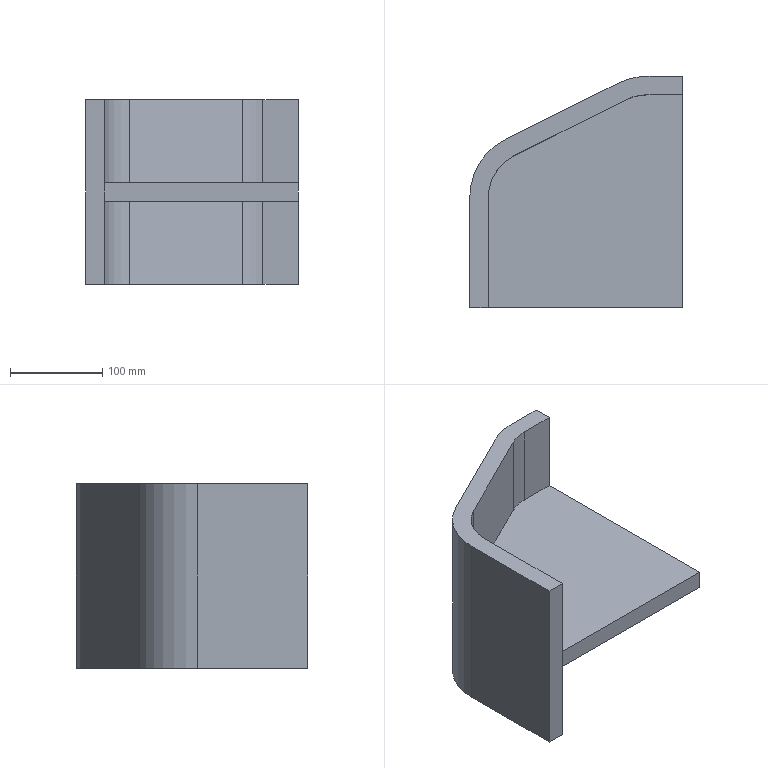Part | SolidWorks | features Extrusion 1, ICE 1 | 2 solids | 23 faces | box 230 x 250 x 200 mm | volume 2385457 mm3 | plane 17 | cylinder 6 | commonest cylinder face diameters 100 x4 140 x2
STEP:
#1=CARTESIAN_POINT('',(0.,119.098,0.));
#2=VERTEX_POINT('',#1);
#3=CARTESIAN_POINT('',(0.,0.,0.));
#4=VERTEX_POINT('',#3);
#5=CARTESIAN_POINT('',(0.,0.,0.));
#6=DIRECTION('',(0.,-1.,0.));
#7=VECTOR('',#6,1000.);
#8=LINE('',#5,#7);
#9=EDGE_CURVE('',#2,#4,#8,.T.);
#10=ORIENTED_EDGE('',*,*,#9,.T.);
#11=CARTESIAN_POINT('',(0.,0.,20.));
#12=VERTEX_POINT('',#11);
#13=CARTESIAN_POINT('',(0.,0.,20.));
#14=DIRECTION('',(0.,0.,-1.));
#15=VECTOR('',#14,1000.);
#16=LINE('',#13,#15);
#17=EDGE_CURVE('',#12,#4,#16,.T.);
#18=ORIENTED_EDGE('',*,*,#17,.F.);
#19=CARTESIAN_POINT('',(0.,119.098,20.));
#20=VERTEX_POINT('',#19);
#21=CARTESIAN_POINT('',(0.,0.,20.));
#22=DIRECTION('',(0.,-1.,0.));
#23=VECTOR('',#22,1000.);
#24=LINE('',#21,#23);
#25=EDGE_CURVE('',#20,#12,#24,.T.);
#26=ORIENTED_EDGE('',*,*,#25,.F.);
#27=CARTESIAN_POINT('',(0.,119.098,20.));
#28=DIRECTION('',(0.,0.,-1.));
#29=VECTOR('',#28,1000.);
#30=LINE('',#27,#29);
#31=EDGE_CURVE('',#20,#2,#30,.T.);
#32=ORIENTED_EDGE('',*,*,#31,.T.);
#33=EDGE_LOOP('',(#10,#18,#26,#32));
#34=FACE_OUTER_BOUND('',#33,.T.);
#35=CARTESIAN_POINT('',(0.,0.,20.));
#36=DIRECTION('',(1.,0.,0.));
#37=DIRECTION('',(0.,0.,-1.));
#38=AXIS2_PLACEMENT_3D('',#35,#36,#37);
#39=PLANE('',#38);
#40=ADVANCED_FACE('',(#34),#39,.F.);
#41=CARTESIAN_POINT('',(210.,0.,0.));
#42=VERTEX_POINT('',#41);
#43=CARTESIAN_POINT('',(0.,0.,0.));
#44=DIRECTION('',(1.,0.,0.));
#45=VECTOR('',#44,1000.);
#46=LINE('',#43,#45);
#47=EDGE_CURVE('',#4,#42,#46,.T.);
#48=ORIENTED_EDGE('',*,*,#47,.T.);
#49=CARTESIAN_POINT('',(210.,0.,20.));
#50=VERTEX_POINT('',#49);
#51=CARTESIAN_POINT('',(210.,0.,20.));
#52=DIRECTION('',(0.,0.,-1.));
#53=VECTOR('',#52,1000.);
#54=LINE('',#51,#53);
#55=EDGE_CURVE('',#50,#42,#54,.T.);
#56=ORIENTED_EDGE('',*,*,#55,.F.);
#57=CARTESIAN_POINT('',(0.,0.,20.));
#58=DIRECTION('',(1.,0.,0.));
#59=VECTOR('',#58,1000.);
#60=LINE('',#57,#59);
#61=EDGE_CURVE('',#12,#50,#60,.T.);
#62=ORIENTED_EDGE('',*,*,#61,.F.);
#63=ORIENTED_EDGE('',*,*,#17,.T.);
#64=EDGE_LOOP('',(#48,#56,#62,#63));
#65=FACE_OUTER_BOUND('',#64,.T.);
#66=CARTESIAN_POINT('',(0.,0.,20.));
#67=DIRECTION('',(0.,1.,0.));
#68=DIRECTION('',(0.,0.,1.));
#69=AXIS2_PLACEMENT_3D('',#66,#67,#68);
#70=PLANE('',#69);
#71=ADVANCED_FACE('',(#65),#70,.F.);
#72=CARTESIAN_POINT('',(210.,230.,0.));
#73=VERTEX_POINT('',#72);
#74=CARTESIAN_POINT('',(210.,230.,0.));
#75=DIRECTION('',(0.,1.,0.));
#76=VECTOR('',#75,1000.);
#77=LINE('',#74,#76);
#78=EDGE_CURVE('',#42,#73,#77,.T.);
#79=ORIENTED_EDGE('',*,*,#78,.T.);
#80=CARTESIAN_POINT('',(210.,230.,20.));
#81=VERTEX_POINT('',#80);
#82=CARTESIAN_POINT('',(210.,230.,20.));
#83=DIRECTION('',(0.,0.,-1.));
#84=VECTOR('',#83,1000.);
#85=LINE('',#82,#84);
#86=EDGE_CURVE('',#81,#73,#85,.T.);
#87=ORIENTED_EDGE('',*,*,#86,.F.);
#88=CARTESIAN_POINT('',(210.,230.,20.));
#89=DIRECTION('',(0.,1.,0.));
#90=VECTOR('',#89,1000.);
#91=LINE('',#88,#90);
#92=EDGE_CURVE('',#50,#81,#91,.T.);
#93=ORIENTED_EDGE('',*,*,#92,.F.);
#94=ORIENTED_EDGE('',*,*,#55,.T.);
#95=EDGE_LOOP('',(#79,#87,#93,#94));
#96=FACE_OUTER_BOUND('',#95,.T.);
#97=CARTESIAN_POINT('',(210.,230.,20.));
#98=DIRECTION('',(-1.,0.,0.));
#99=DIRECTION('',(0.,-1.,0.));
#100=AXIS2_PLACEMENT_3D('',#97,#98,#99);
#101=PLANE('',#100);
#102=ADVANCED_FACE('',(#96),#101,.F.);
#103=CARTESIAN_POINT('',(171.803,230.,0.));
#104=VERTEX_POINT('',#103);
#105=CARTESIAN_POINT('',(171.803,230.,0.));
#106=DIRECTION('',(-1.,0.,0.));
#107=VECTOR('',#106,1000.);
#108=LINE('',#105,#107);
#109=EDGE_CURVE('',#73,#104,#108,.T.);
#110=ORIENTED_EDGE('',*,*,#109,.T.);
#111=CARTESIAN_POINT('',(171.803,230.,20.));
#112=VERTEX_POINT('',#111);
#113=CARTESIAN_POINT('',(171.803,230.,20.));
#114=DIRECTION('',(0.,0.,-1.));
#115=VECTOR('',#114,1000.);
#116=LINE('',#113,#115);
#117=EDGE_CURVE('',#112,#104,#116,.T.);
#118=ORIENTED_EDGE('',*,*,#117,.F.);
#119=CARTESIAN_POINT('',(171.803,230.,20.));
#120=DIRECTION('',(-1.,0.,0.));
#121=VECTOR('',#120,1000.);
#122=LINE('',#119,#121);
#123=EDGE_CURVE('',#81,#112,#122,.T.);
#124=ORIENTED_EDGE('',*,*,#123,.F.);
#125=ORIENTED_EDGE('',*,*,#86,.T.);
#126=EDGE_LOOP('',(#110,#118,#124,#125));
#127=FACE_OUTER_BOUND('',#126,.T.);
#128=CARTESIAN_POINT('',(171.803,230.,20.));
#129=DIRECTION('',(0.,-1.,0.));
#130=DIRECTION('',(0.,0.,-1.));
#131=AXIS2_PLACEMENT_3D('',#128,#129,#130);
#132=PLANE('',#131);
#133=ADVANCED_FACE('',(#127),#132,.F.);
#134=CARTESIAN_POINT('',(149.443,224.721,0.));
#135=VERTEX_POINT('',#134);
#136=CARTESIAN_POINT('',(171.803,180.,0.));
#137=DIRECTION('',(0.,0.,1.));
#138=DIRECTION('',(-1.,0.,0.));
#139=AXIS2_PLACEMENT_3D('',#136,#137,#138);
#140=CIRCLE('',#139,50.);
#141=EDGE_CURVE('',#104,#135,#140,.T.);
#142=ORIENTED_EDGE('',*,*,#141,.T.);
#143=CARTESIAN_POINT('',(149.443,224.721,20.));
#144=VERTEX_POINT('',#143);
#145=CARTESIAN_POINT('',(149.443,224.721,20.));
#146=DIRECTION('',(0.,0.,-1.));
#147=VECTOR('',#146,1000.);
#148=LINE('',#145,#147);
#149=EDGE_CURVE('',#144,#135,#148,.T.);
#150=ORIENTED_EDGE('',*,*,#149,.F.);
#151=CARTESIAN_POINT('',(171.803,180.,20.));
#152=DIRECTION('',(0.,0.,1.));
#153=DIRECTION('',(-1.,0.,0.));
#154=AXIS2_PLACEMENT_3D('',#151,#152,#153);
#155=CIRCLE('',#154,50.);
#156=EDGE_CURVE('',#112,#144,#155,.T.);
#157=ORIENTED_EDGE('',*,*,#156,.F.);
#158=ORIENTED_EDGE('',*,*,#117,.T.);
#159=EDGE_LOOP('',(#142,#150,#157,#158));
#160=FACE_OUTER_BOUND('',#159,.T.);
#161=CARTESIAN_POINT('',(171.803,180.,20.));
#162=DIRECTION('',(0.,0.,-1.));
#163=DIRECTION('',(-1.,0.,0.));
#164=AXIS2_PLACEMENT_3D('',#161,#162,#163);
#165=CYLINDRICAL_SURFACE('',#164,50.);
#166=ADVANCED_FACE('',(#160),#165,.T.);
#167=CARTESIAN_POINT('',(27.639,163.82,0.));
#168=VERTEX_POINT('',#167);
#169=CARTESIAN_POINT('',(149.443,224.721,0.));
#170=DIRECTION('',(-0.8944,-0.4472,0.));
#171=VECTOR('',#170,1000.);
#172=LINE('',#169,#171);
#173=EDGE_CURVE('',#135,#168,#172,.T.);
#174=ORIENTED_EDGE('',*,*,#173,.T.);
#175=CARTESIAN_POINT('',(27.639,163.82,20.));
#176=VERTEX_POINT('',#175);
#177=CARTESIAN_POINT('',(27.639,163.82,20.));
#178=DIRECTION('',(0.,0.,-1.));
#179=VECTOR('',#178,1000.);
#180=LINE('',#177,#179);
#181=EDGE_CURVE('',#176,#168,#180,.T.);
#182=ORIENTED_EDGE('',*,*,#181,.F.);
#183=CARTESIAN_POINT('',(149.443,224.721,20.));
#184=DIRECTION('',(-0.8944,-0.4472,0.));
#185=VECTOR('',#184,1000.);
#186=LINE('',#183,#185);
#187=EDGE_CURVE('',#144,#176,#186,.T.);
#188=ORIENTED_EDGE('',*,*,#187,.F.);
#189=ORIENTED_EDGE('',*,*,#149,.T.);
#190=EDGE_LOOP('',(#174,#182,#188,#189));
#191=FACE_OUTER_BOUND('',#190,.T.);
#192=CARTESIAN_POINT('',(149.443,224.721,20.));
#193=DIRECTION('',(0.4472,-0.8944,0.));
#194=DIRECTION('',(0.8944,0.4472,0.));
#195=AXIS2_PLACEMENT_3D('',#192,#193,#194);
#196=PLANE('',#195);
#197=ADVANCED_FACE('',(#191),#196,.F.);
#198=CARTESIAN_POINT('',(50.,119.098,0.));
#199=DIRECTION('',(0.,0.,1.));
#200=DIRECTION('',(-1.,0.,0.));
#201=AXIS2_PLACEMENT_3D('',#198,#199,#200);
#202=CIRCLE('',#201,50.);
#203=EDGE_CURVE('',#168,#2,#202,.T.);
#204=ORIENTED_EDGE('',*,*,#203,.T.);
#205=ORIENTED_EDGE('',*,*,#31,.F.);
#206=CARTESIAN_POINT('',(50.,119.098,20.));
#207=DIRECTION('',(0.,0.,1.));
#208=DIRECTION('',(-1.,0.,0.));
#209=AXIS2_PLACEMENT_3D('',#206,#207,#208);
#210=CIRCLE('',#209,50.);
#211=EDGE_CURVE('',#176,#20,#210,.T.);
#212=ORIENTED_EDGE('',*,*,#211,.F.);
#213=ORIENTED_EDGE('',*,*,#181,.T.);
#214=EDGE_LOOP('',(#204,#205,#212,#213));
#215=FACE_OUTER_BOUND('',#214,.T.);
#216=CARTESIAN_POINT('',(50.,119.098,20.));
#217=DIRECTION('',(0.,0.,-1.));
#218=DIRECTION('',(-1.,0.,0.));
#219=AXIS2_PLACEMENT_3D('',#216,#217,#218);
#220=CYLINDRICAL_SURFACE('',#219,50.);
#221=ADVANCED_FACE('',(#215),#220,.T.);
#222=ORIENTED_EDGE('',*,*,#25,.T.);
#223=ORIENTED_EDGE('',*,*,#61,.T.);
#224=ORIENTED_EDGE('',*,*,#92,.T.);
#225=ORIENTED_EDGE('',*,*,#123,.T.);
#226=ORIENTED_EDGE('',*,*,#156,.T.);
#227=ORIENTED_EDGE('',*,*,#187,.T.);
#228=ORIENTED_EDGE('',*,*,#211,.T.);
#229=EDGE_LOOP('',(#222,#223,#224,#225,#226,#227,#228));
#230=FACE_OUTER_BOUND('',#229,.T.);
#231=CARTESIAN_POINT('',(50.,119.098,20.));
#232=DIRECTION('',(0.,0.,-1.));
#233=DIRECTION('',(-1.,0.,0.));
#234=AXIS2_PLACEMENT_3D('',#231,#232,#233);
#235=PLANE('',#234);
#236=ADVANCED_FACE('',(#230),#235,.F.);
#237=ORIENTED_EDGE('',*,*,#9,.F.);
#238=ORIENTED_EDGE('',*,*,#203,.F.);
#239=ORIENTED_EDGE('',*,*,#173,.F.);
#240=ORIENTED_EDGE('',*,*,#141,.F.);
#241=ORIENTED_EDGE('',*,*,#109,.F.);
#242=ORIENTED_EDGE('',*,*,#78,.F.);
#243=ORIENTED_EDGE('',*,*,#47,.F.);
#244=EDGE_LOOP('',(#237,#238,#239,#240,#241,#242,#243));
#245=FACE_OUTER_BOUND('',#244,.T.);
#246=CARTESIAN_POINT('',(50.,119.098,0.));
#247=DIRECTION('',(0.,0.,-1.));
#248=DIRECTION('',(-1.,0.,0.));
#249=AXIS2_PLACEMENT_3D('',#246,#247,#248);
#250=PLANE('',#249);
#251=ADVANCED_FACE('',(#245),#250,.T.);
#252=CLOSED_SHELL('',(#40,#71,#102,#133,#166,#197,#221,#236,#251));
#253=MANIFOLD_SOLID_BREP('',#252);
#254=CARTESIAN_POINT('',(0.,119.098,-90.));
#255=VERTEX_POINT('',#254);
#256=CARTESIAN_POINT('',(27.639,163.82,-90.));
#257=VERTEX_POINT('',#256);
#258=CARTESIAN_POINT('',(50.,119.098,-90.));
#259=DIRECTION('',(0.,0.,-1.));
#260=DIRECTION('',(1.,0.,0.));
#261=AXIS2_PLACEMENT_3D('',#258,#259,#260);
#262=CIRCLE('',#261,50.);
#263=EDGE_CURVE('',#255,#257,#262,.T.);
#264=ORIENTED_EDGE('',*,*,#263,.T.);
#265=CARTESIAN_POINT('',(27.639,163.82,110.));
#266=VERTEX_POINT('',#265);
#267=CARTESIAN_POINT('',(27.639,163.82,110.));
#268=DIRECTION('',(0.,0.,-1.));
#269=VECTOR('',#268,1000.);
#270=LINE('',#267,#269);
#271=EDGE_CURVE('',#266,#257,#270,.T.);
#272=ORIENTED_EDGE('',*,*,#271,.F.);
#273=CARTESIAN_POINT('',(0.,119.098,110.));
#274=VERTEX_POINT('',#273);
#275=CARTESIAN_POINT('',(50.,119.098,110.));
#276=DIRECTION('',(0.,0.,-1.));
#277=DIRECTION('',(1.,0.,0.));
#278=AXIS2_PLACEMENT_3D('',#275,#276,#277);
#279=CIRCLE('',#278,50.);
#280=EDGE_CURVE('',#274,#266,#279,.T.);
#281=ORIENTED_EDGE('',*,*,#280,.F.);
#282=CARTESIAN_POINT('',(0.,119.098,110.));
#283=DIRECTION('',(0.,0.,-1.));
#284=VECTOR('',#283,1000.);
#285=LINE('',#282,#284);
#286=EDGE_CURVE('',#274,#255,#285,.T.);
#287=ORIENTED_EDGE('',*,*,#286,.T.);
#288=EDGE_LOOP('',(#264,#272,#281,#287));
#289=FACE_OUTER_BOUND('',#288,.T.);
#290=CARTESIAN_POINT('',(50.,119.098,110.));
#291=DIRECTION('',(0.,0.,-1.));
#292=DIRECTION('',(-1.,0.,0.));
#293=AXIS2_PLACEMENT_3D('',#290,#291,#292);
#294=CYLINDRICAL_SURFACE('',#293,50.);
#295=ADVANCED_FACE('',(#289),#294,.F.);
#296=CARTESIAN_POINT('',(149.443,224.721,-90.));
#297=VERTEX_POINT('',#296);
#298=CARTESIAN_POINT('',(149.443,224.721,-90.));
#299=DIRECTION('',(0.8944,0.4472,0.));
#300=VECTOR('',#299,1000.);
#301=LINE('',#298,#300);
#302=EDGE_CURVE('',#257,#297,#301,.T.);
#303=ORIENTED_EDGE('',*,*,#302,.T.);
#304=CARTESIAN_POINT('',(149.443,224.721,110.));
#305=VERTEX_POINT('',#304);
#306=CARTESIAN_POINT('',(149.443,224.721,110.));
#307=DIRECTION('',(0.,0.,-1.));
#308=VECTOR('',#307,1000.);
#309=LINE('',#306,#308);
#310=EDGE_CURVE('',#305,#297,#309,.T.);
#311=ORIENTED_EDGE('',*,*,#310,.F.);
#312=CARTESIAN_POINT('',(149.443,224.721,110.));
#313=DIRECTION('',(0.8944,0.4472,0.));
#314=VECTOR('',#313,1000.);
#315=LINE('',#312,#314);
#316=EDGE_CURVE('',#266,#305,#315,.T.);
#317=ORIENTED_EDGE('',*,*,#316,.F.);
#318=ORIENTED_EDGE('',*,*,#271,.T.);
#319=EDGE_LOOP('',(#303,#311,#317,#318));
#320=FACE_OUTER_BOUND('',#319,.T.);
#321=CARTESIAN_POINT('',(149.443,224.721,110.));
#322=DIRECTION('',(-0.4472,0.8944,0.));
#323=DIRECTION('',(-0.8944,-0.4472,0.));
#324=AXIS2_PLACEMENT_3D('',#321,#322,#323);
#325=PLANE('',#324);
#326=ADVANCED_FACE('',(#320),#325,.F.);
#327=CARTESIAN_POINT('',(171.803,230.,-90.));
#328=VERTEX_POINT('',#327);
#329=CARTESIAN_POINT('',(171.803,180.,-90.));
#330=DIRECTION('',(0.,0.,-1.));
#331=DIRECTION('',(1.,0.,0.));
#332=AXIS2_PLACEMENT_3D('',#329,#330,#331);
#333=CIRCLE('',#332,50.);
#334=EDGE_CURVE('',#297,#328,#333,.T.);
#335=ORIENTED_EDGE('',*,*,#334,.T.);
#336=CARTESIAN_POINT('',(171.803,230.,110.));
#337=VERTEX_POINT('',#336);
#338=CARTESIAN_POINT('',(171.803,230.,110.));
#339=DIRECTION('',(0.,0.,-1.));
#340=VECTOR('',#339,1000.);
#341=LINE('',#338,#340);
#342=EDGE_CURVE('',#337,#328,#341,.T.);
#343=ORIENTED_EDGE('',*,*,#342,.F.);
#344=CARTESIAN_POINT('',(171.803,180.,110.));
#345=DIRECTION('',(0.,0.,-1.));
#346=DIRECTION('',(1.,0.,0.));
#347=AXIS2_PLACEMENT_3D('',#344,#345,#346);
#348=CIRCLE('',#347,50.);
#349=EDGE_CURVE('',#305,#337,#348,.T.);
#350=ORIENTED_EDGE('',*,*,#349,.F.);
#351=ORIENTED_EDGE('',*,*,#310,.T.);
#352=EDGE_LOOP('',(#335,#343,#350,#351));
#353=FACE_OUTER_BOUND('',#352,.T.);
#354=CARTESIAN_POINT('',(171.803,180.,110.));
#355=DIRECTION('',(0.,0.,-1.));
#356=DIRECTION('',(-1.,0.,0.));
#357=AXIS2_PLACEMENT_3D('',#354,#355,#356);
#358=CYLINDRICAL_SURFACE('',#357,50.);
#359=ADVANCED_FACE('',(#353),#358,.F.);
#360=CARTESIAN_POINT('',(210.,230.,-90.));
#361=VERTEX_POINT('',#360);
#362=CARTESIAN_POINT('',(210.,230.,-90.));
#363=DIRECTION('',(1.,0.,0.));
#364=VECTOR('',#363,1000.);
#365=LINE('',#362,#364);
#366=EDGE_CURVE('',#328,#361,#365,.T.);
#367=ORIENTED_EDGE('',*,*,#366,.T.);
#368=CARTESIAN_POINT('',(210.,230.,110.));
#369=VERTEX_POINT('',#368);
#370=CARTESIAN_POINT('',(210.,230.,110.));
#371=DIRECTION('',(0.,0.,-1.));
#372=VECTOR('',#371,1000.);
#373=LINE('',#370,#372);
#374=EDGE_CURVE('',#369,#361,#373,.T.);
#375=ORIENTED_EDGE('',*,*,#374,.F.);
#376=CARTESIAN_POINT('',(210.,230.,110.));
#377=DIRECTION('',(1.,0.,0.));
#378=VECTOR('',#377,1000.);
#379=LINE('',#376,#378);
#380=EDGE_CURVE('',#337,#369,#379,.T.);
#381=ORIENTED_EDGE('',*,*,#380,.F.);
#382=ORIENTED_EDGE('',*,*,#342,.T.);
#383=EDGE_LOOP('',(#367,#375,#381,#382));
#384=FACE_OUTER_BOUND('',#383,.T.);
#385=CARTESIAN_POINT('',(210.,230.,110.));
#386=DIRECTION('',(0.,1.,0.));
#387=DIRECTION('',(0.,0.,1.));
#388=AXIS2_PLACEMENT_3D('',#385,#386,#387);
#389=PLANE('',#388);
#390=ADVANCED_FACE('',(#384),#389,.F.);
#391=CARTESIAN_POINT('',(210.,250.,-90.));
#392=VERTEX_POINT('',#391);
#393=CARTESIAN_POINT('',(210.,250.,-90.));
#394=DIRECTION('',(0.,1.,0.));
#395=VECTOR('',#394,1000.);
#396=LINE('',#393,#395);
#397=EDGE_CURVE('',#361,#392,#396,.T.);
#398=ORIENTED_EDGE('',*,*,#397,.T.);
#399=CARTESIAN_POINT('',(210.,250.,110.));
#400=VERTEX_POINT('',#399);
#401=CARTESIAN_POINT('',(210.,250.,110.));
#402=DIRECTION('',(0.,0.,-1.));
#403=VECTOR('',#402,1000.);
#404=LINE('',#401,#403);
#405=EDGE_CURVE('',#400,#392,#404,.T.);
#406=ORIENTED_EDGE('',*,*,#405,.F.);
#407=CARTESIAN_POINT('',(210.,250.,110.));
#408=DIRECTION('',(0.,1.,0.));
#409=VECTOR('',#408,1000.);
#410=LINE('',#407,#409);
#411=EDGE_CURVE('',#369,#400,#410,.T.);
#412=ORIENTED_EDGE('',*,*,#411,.F.);
#413=ORIENTED_EDGE('',*,*,#374,.T.);
#414=EDGE_LOOP('',(#398,#406,#412,#413));
#415=FACE_OUTER_BOUND('',#414,.T.);
#416=CARTESIAN_POINT('',(210.,250.,110.));
#417=DIRECTION('',(-1.,0.,0.));
#418=DIRECTION('',(0.,0.,1.));
#419=AXIS2_PLACEMENT_3D('',#416,#417,#418);
#420=PLANE('',#419);
#421=ADVANCED_FACE('',(#415),#420,.F.);
#422=CARTESIAN_POINT('',(171.803,250.,-90.));
#423=VERTEX_POINT('',#422);
#424=CARTESIAN_POINT('',(210.,250.,-90.));
#425=DIRECTION('',(-1.,0.,0.));
#426=VECTOR('',#425,1000.);
#427=LINE('',#424,#426);
#428=EDGE_CURVE('',#392,#423,#427,.T.);
#429=ORIENTED_EDGE('',*,*,#428,.T.);
#430=CARTESIAN_POINT('',(171.803,250.,110.));
#431=VERTEX_POINT('',#430);
#432=CARTESIAN_POINT('',(171.803,250.,110.));
#433=DIRECTION('',(0.,0.,-1.));
#434=VECTOR('',#433,1000.);
#435=LINE('',#432,#434);
#436=EDGE_CURVE('',#431,#423,#435,.T.);
#437=ORIENTED_EDGE('',*,*,#436,.F.);
#438=CARTESIAN_POINT('',(210.,250.,110.));
#439=DIRECTION('',(-1.,0.,0.));
#440=VECTOR('',#439,1000.);
#441=LINE('',#438,#440);
#442=EDGE_CURVE('',#400,#431,#441,.T.);
#443=ORIENTED_EDGE('',*,*,#442,.F.);
#444=ORIENTED_EDGE('',*,*,#405,.T.);
#445=EDGE_LOOP('',(#429,#437,#443,#444));
#446=FACE_OUTER_BOUND('',#445,.T.);
#447=CARTESIAN_POINT('',(210.,250.,110.));
#448=DIRECTION('',(0.,-1.,0.));
#449=DIRECTION('',(0.,0.,-1.));
#450=AXIS2_PLACEMENT_3D('',#447,#448,#449);
#451=PLANE('',#450);
#452=ADVANCED_FACE('',(#446),#451,.F.);
#453=CARTESIAN_POINT('',(140.498,242.61,-90.));
#454=VERTEX_POINT('',#453);
#455=CARTESIAN_POINT('',(171.803,180.,-90.));
#456=DIRECTION('',(0.,0.,1.));
#457=DIRECTION('',(1.,0.,0.));
#458=AXIS2_PLACEMENT_3D('',#455,#456,#457);
#459=CIRCLE('',#458,70.);
#460=EDGE_CURVE('',#423,#454,#459,.T.);
#461=ORIENTED_EDGE('',*,*,#460,.T.);
#462=CARTESIAN_POINT('',(140.498,242.61,110.));
#463=VERTEX_POINT('',#462);
#464=CARTESIAN_POINT('',(140.498,242.61,110.));
#465=DIRECTION('',(0.,0.,-1.));
#466=VECTOR('',#465,1000.);
#467=LINE('',#464,#466);
#468=EDGE_CURVE('',#463,#454,#467,.T.);
#469=ORIENTED_EDGE('',*,*,#468,.F.);
#470=CARTESIAN_POINT('',(171.803,180.,110.));
#471=DIRECTION('',(0.,0.,1.));
#472=DIRECTION('',(1.,0.,0.));
#473=AXIS2_PLACEMENT_3D('',#470,#471,#472);
#474=CIRCLE('',#473,70.);
#475=EDGE_CURVE('',#431,#463,#474,.T.);
#476=ORIENTED_EDGE('',*,*,#475,.F.);
#477=ORIENTED_EDGE('',*,*,#436,.T.);
#478=EDGE_LOOP('',(#461,#469,#476,#477));
#479=FACE_OUTER_BOUND('',#478,.T.);
#480=CARTESIAN_POINT('',(171.803,180.,110.));
#481=DIRECTION('',(0.,0.,-1.));
#482=DIRECTION('',(-1.,0.,0.));
#483=AXIS2_PLACEMENT_3D('',#480,#481,#482);
#484=CYLINDRICAL_SURFACE('',#483,70.);
#485=ADVANCED_FACE('',(#479),#484,.T.);
#486=CARTESIAN_POINT('',(18.695,181.708,-90.));
#487=VERTEX_POINT('',#486);
#488=CARTESIAN_POINT('',(140.498,242.61,-90.));
#489=DIRECTION('',(-0.8944,-0.4472,0.));
#490=VECTOR('',#489,1000.);
#491=LINE('',#488,#490);
#492=EDGE_CURVE('',#454,#487,#491,.T.);
#493=ORIENTED_EDGE('',*,*,#492,.T.);
#494=CARTESIAN_POINT('',(18.695,181.708,110.));
#495=VERTEX_POINT('',#494);
#496=CARTESIAN_POINT('',(18.695,181.708,110.));
#497=DIRECTION('',(0.,0.,-1.));
#498=VECTOR('',#497,1000.);
#499=LINE('',#496,#498);
#500=EDGE_CURVE('',#495,#487,#499,.T.);
#501=ORIENTED_EDGE('',*,*,#500,.F.);
#502=CARTESIAN_POINT('',(140.498,242.61,110.));
#503=DIRECTION('',(-0.8944,-0.4472,0.));
#504=VECTOR('',#503,1000.);
#505=LINE('',#502,#504);
#506=EDGE_CURVE('',#463,#495,#505,.T.);
#507=ORIENTED_EDGE('',*,*,#506,.F.);
#508=ORIENTED_EDGE('',*,*,#468,.T.);
#509=EDGE_LOOP('',(#493,#501,#507,#508));
#510=FACE_OUTER_BOUND('',#509,.T.);
#511=CARTESIAN_POINT('',(140.498,242.61,110.));
#512=DIRECTION('',(0.4472,-0.8944,0.));
#513=DIRECTION('',(0.8944,0.4472,0.));
#514=AXIS2_PLACEMENT_3D('',#511,#512,#513);
#515=PLANE('',#514);
#516=ADVANCED_FACE('',(#510),#515,.F.);
#517=CARTESIAN_POINT('',(-20.,119.098,-90.));
#518=VERTEX_POINT('',#517);
#519=CARTESIAN_POINT('',(50.,119.098,-90.));
#520=DIRECTION('',(0.,0.,1.));
#521=DIRECTION('',(1.,0.,0.));
#522=AXIS2_PLACEMENT_3D('',#519,#520,#521);
#523=CIRCLE('',#522,70.);
#524=EDGE_CURVE('',#487,#518,#523,.T.);
#525=ORIENTED_EDGE('',*,*,#524,.T.);
#526=CARTESIAN_POINT('',(-20.,119.098,110.));
#527=VERTEX_POINT('',#526);
#528=CARTESIAN_POINT('',(-20.,119.098,110.));
#529=DIRECTION('',(0.,0.,-1.));
#530=VECTOR('',#529,1000.);
#531=LINE('',#528,#530);
#532=EDGE_CURVE('',#527,#518,#531,.T.);
#533=ORIENTED_EDGE('',*,*,#532,.F.);
#534=CARTESIAN_POINT('',(50.,119.098,110.));
#535=DIRECTION('',(0.,0.,1.));
#536=DIRECTION('',(1.,0.,0.));
#537=AXIS2_PLACEMENT_3D('',#534,#535,#536);
#538=CIRCLE('',#537,70.);
#539=EDGE_CURVE('',#495,#527,#538,.T.);
#540=ORIENTED_EDGE('',*,*,#539,.F.);
#541=ORIENTED_EDGE('',*,*,#500,.T.);
#542=EDGE_LOOP('',(#525,#533,#540,#541));
#543=FACE_OUTER_BOUND('',#542,.T.);
#544=CARTESIAN_POINT('',(50.,119.098,110.));
#545=DIRECTION('',(0.,0.,-1.));
#546=DIRECTION('',(-1.,0.,0.));
#547=AXIS2_PLACEMENT_3D('',#544,#545,#546);
#548=CYLINDRICAL_SURFACE('',#547,70.);
#549=ADVANCED_FACE('',(#543),#548,.T.);
#550=CARTESIAN_POINT('',(-20.,0.,-90.));
#551=VERTEX_POINT('',#550);
#552=CARTESIAN_POINT('',(-20.,119.098,-90.));
#553=DIRECTION('',(0.,-1.,0.));
#554=VECTOR('',#553,1000.);
#555=LINE('',#552,#554);
#556=EDGE_CURVE('',#518,#551,#555,.T.);
#557=ORIENTED_EDGE('',*,*,#556,.T.);
#558=CARTESIAN_POINT('',(-20.,0.,110.));
#559=VERTEX_POINT('',#558);
#560=CARTESIAN_POINT('',(-20.,0.,110.));
#561=DIRECTION('',(0.,0.,-1.));
#562=VECTOR('',#561,1000.);
#563=LINE('',#560,#562);
#564=EDGE_CURVE('',#559,#551,#563,.T.);
#565=ORIENTED_EDGE('',*,*,#564,.F.);
#566=CARTESIAN_POINT('',(-20.,119.098,110.));
#567=DIRECTION('',(0.,-1.,0.));
#568=VECTOR('',#567,1000.);
#569=LINE('',#566,#568);
#570=EDGE_CURVE('',#527,#559,#569,.T.);
#571=ORIENTED_EDGE('',*,*,#570,.F.);
#572=ORIENTED_EDGE('',*,*,#532,.T.);
#573=EDGE_LOOP('',(#557,#565,#571,#572));
#574=FACE_OUTER_BOUND('',#573,.T.);
#575=CARTESIAN_POINT('',(-20.,119.098,110.));
#576=DIRECTION('',(1.,0.,0.));
#577=DIRECTION('',(0.,1.,0.));
#578=AXIS2_PLACEMENT_3D('',#575,#576,#577);
#579=PLANE('',#578);
#580=ADVANCED_FACE('',(#574),#579,.F.);
#581=CARTESIAN_POINT('',(0.,0.,-90.));
#582=VERTEX_POINT('',#581);
#583=CARTESIAN_POINT('',(0.,0.,-90.));
#584=DIRECTION('',(1.,0.,0.));
#585=VECTOR('',#584,1000.);
#586=LINE('',#583,#585);
#587=EDGE_CURVE('',#551,#582,#586,.T.);
#588=ORIENTED_EDGE('',*,*,#587,.T.);
#589=CARTESIAN_POINT('',(0.,0.,110.));
#590=VERTEX_POINT('',#589);
#591=CARTESIAN_POINT('',(0.,0.,110.));
#592=DIRECTION('',(0.,0.,-1.));
#593=VECTOR('',#592,1000.);
#594=LINE('',#591,#593);
#595=EDGE_CURVE('',#590,#582,#594,.T.);
#596=ORIENTED_EDGE('',*,*,#595,.F.);
#597=CARTESIAN_POINT('',(0.,0.,110.));
#598=DIRECTION('',(1.,0.,0.));
#599=VECTOR('',#598,1000.);
#600=LINE('',#597,#599);
#601=EDGE_CURVE('',#559,#590,#600,.T.);
#602=ORIENTED_EDGE('',*,*,#601,.F.);
#603=ORIENTED_EDGE('',*,*,#564,.T.);
#604=EDGE_LOOP('',(#588,#596,#602,#603));
#605=FACE_OUTER_BOUND('',#604,.T.);
#606=CARTESIAN_POINT('',(0.,0.,110.));
#607=DIRECTION('',(0.,1.,0.));
#608=DIRECTION('',(-1.,0.,0.));
#609=AXIS2_PLACEMENT_3D('',#606,#607,#608);
#610=PLANE('',#609);
#611=ADVANCED_FACE('',(#605),#610,.F.);
#612=CARTESIAN_POINT('',(0.,119.098,-90.));
#613=DIRECTION('',(0.,1.,0.));
#614=VECTOR('',#613,1000.);
#615=LINE('',#612,#614);
#616=EDGE_CURVE('',#582,#255,#615,.T.);
#617=ORIENTED_EDGE('',*,*,#616,.T.);
#618=ORIENTED_EDGE('',*,*,#286,.F.);
#619=CARTESIAN_POINT('',(0.,119.098,110.));
#620=DIRECTION('',(0.,1.,0.));
#621=VECTOR('',#620,1000.);
#622=LINE('',#619,#621);
#623=EDGE_CURVE('',#590,#274,#622,.T.);
#624=ORIENTED_EDGE('',*,*,#623,.F.);
#625=ORIENTED_EDGE('',*,*,#595,.T.);
#626=EDGE_LOOP('',(#617,#618,#624,#625));
#627=FACE_OUTER_BOUND('',#626,.T.);
#628=CARTESIAN_POINT('',(0.,119.098,110.));
#629=DIRECTION('',(-1.,0.,0.));
#630=DIRECTION('',(0.,-1.,0.));
#631=AXIS2_PLACEMENT_3D('',#628,#629,#630);
#632=PLANE('',#631);
#633=ADVANCED_FACE('',(#627),#632,.F.);
#634=ORIENTED_EDGE('',*,*,#280,.T.);
#635=ORIENTED_EDGE('',*,*,#316,.T.);
#636=ORIENTED_EDGE('',*,*,#349,.T.);
#637=ORIENTED_EDGE('',*,*,#380,.T.);
#638=ORIENTED_EDGE('',*,*,#411,.T.);
#639=ORIENTED_EDGE('',*,*,#442,.T.);
#640=ORIENTED_EDGE('',*,*,#475,.T.);
#641=ORIENTED_EDGE('',*,*,#506,.T.);
#642=ORIENTED_EDGE('',*,*,#539,.T.);
#643=ORIENTED_EDGE('',*,*,#570,.T.);
#644=ORIENTED_EDGE('',*,*,#601,.T.);
#645=ORIENTED_EDGE('',*,*,#623,.T.);
#646=EDGE_LOOP('',(#634,#635,#636,#637,#638,#639,#640,#641,#642,#643,#644,#645));
#647=FACE_OUTER_BOUND('',#646,.T.);
#648=CARTESIAN_POINT('',(50.,119.098,110.));
#649=DIRECTION('',(0.,0.,1.));
#650=DIRECTION('',(1.,0.,0.));
#651=AXIS2_PLACEMENT_3D('',#648,#649,#650);
#652=PLANE('',#651);
#653=ADVANCED_FACE('',(#647),#652,.T.);
#654=ORIENTED_EDGE('',*,*,#263,.F.);
#655=ORIENTED_EDGE('',*,*,#616,.F.);
#656=ORIENTED_EDGE('',*,*,#587,.F.);
#657=ORIENTED_EDGE('',*,*,#556,.F.);
#658=ORIENTED_EDGE('',*,*,#524,.F.);
#659=ORIENTED_EDGE('',*,*,#492,.F.);
#660=ORIENTED_EDGE('',*,*,#460,.F.);
#661=ORIENTED_EDGE('',*,*,#428,.F.);
#662=ORIENTED_EDGE('',*,*,#397,.F.);
#663=ORIENTED_EDGE('',*,*,#366,.F.);
#664=ORIENTED_EDGE('',*,*,#334,.F.);
#665=ORIENTED_EDGE('',*,*,#302,.F.);
#666=EDGE_LOOP('',(#654,#655,#656,#657,#658,#659,#660,#661,#662,#663,#664,#665));
#667=FACE_OUTER_BOUND('',#666,.T.);
#668=CARTESIAN_POINT('',(50.,119.098,-90.));
#669=DIRECTION('',(0.,0.,1.));
#670=DIRECTION('',(1.,0.,0.));
#671=AXIS2_PLACEMENT_3D('',#668,#669,#670);
#672=PLANE('',#671);
#673=ADVANCED_FACE('',(#667),#672,.F.);
#674=CLOSED_SHELL('',(#295,#326,#359,#390,#421,#452,#485,#516,#549,#580,#611,#633,#653,#673));
#675=MANIFOLD_SOLID_BREP('',#674);
#676=CARTESIAN_POINT('',(0.,0.,0.));
#677=DIRECTION('',(0.,0.,1.));
#678=DIRECTION('',(1.,0.,0.));
#679=AXIS2_PLACEMENT_3D('',#676,#677,#678);
#680=(LENGTH_UNIT()NAMED_UNIT(*)SI_UNIT(.MILLI.,.METRE.));
#681=UNCERTAINTY_MEASURE_WITH_UNIT(LENGTH_MEASURE(0.00001),#680,'','');
#682=(NAMED_UNIT(*)PLANE_ANGLE_UNIT()SI_UNIT($,.RADIAN.));
#683=(NAMED_UNIT(*)SI_UNIT($,.STERADIAN.)SOLID_ANGLE_UNIT());
#684=(GEOMETRIC_REPRESENTATION_CONTEXT(3)GLOBAL_UNCERTAINTY_ASSIGNED_CONTEXT((#681))GLOBAL_UNIT_ASSIGNED_CONTEXT((#680,#682,#683))REPRESENTATION_CONTEXT('',''));
#685=ADVANCED_BREP_SHAPE_REPRESENTATION('',(#253,#675,#679),#684);